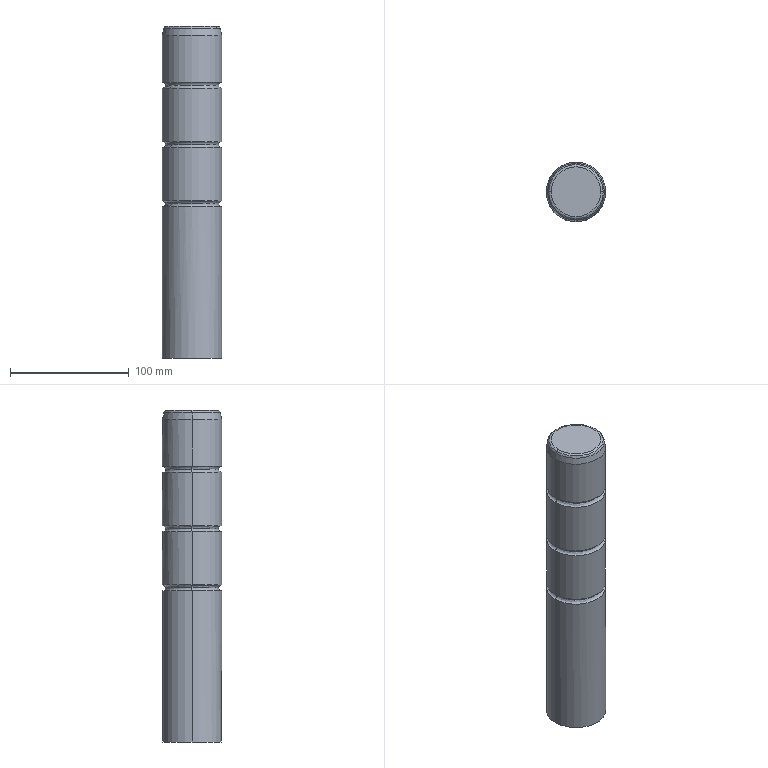Part | Creo | 1 solid | 33 faces | box 50 x 50 x 280 mm | volume 542043 mm3 | torus 16 | cylinder 10 | cone 4 | plane 3 | commonest cylinder face diameters 50 x8 10.579 x2
STEP:
#1=CARTESIAN_POINT('',(0.,0.,0.));
#2=DIRECTION('',(0.,0.,1.));
#3=DIRECTION('',(1.,0.,0.));
#4=AXIS2_PLACEMENT_3D('',#1,#2,#3);
#5=CARTESIAN_POINT('',(-257.899,252.373,-128.441));
#6=VERTEX_POINT('',#5);
#7=CARTESIAN_POINT('',(-307.899,252.373,-128.441));
#8=VERTEX_POINT('',#7);
#9=CARTESIAN_POINT('',(-282.899,252.373,-128.441));
#10=DIRECTION('',(0.,0.,-1.));
#11=DIRECTION('',(1.,0.,0.));
#12=AXIS2_PLACEMENT_3D('',#9,#10,#11);
#13=CIRCLE('',#12,25.);
#14=EDGE_CURVE('',#6,#8,#13,.T.);
#15=ORIENTED_EDGE('',*,*,#14,.F.);
#16=CARTESIAN_POINT('',(-282.899,252.373,-128.441));
#17=DIRECTION('',(0.,0.,-1.));
#18=DIRECTION('',(-1.,0.,0.));
#19=AXIS2_PLACEMENT_3D('',#16,#17,#18);
#20=CIRCLE('',#19,25.);
#21=EDGE_CURVE('',#8,#6,#20,.T.);
#22=ORIENTED_EDGE('',*,*,#21,.F.);
#23=EDGE_LOOP('',(#15,#22));
#24=FACE_OUTER_BOUND('',#23,.F.);
#25=CARTESIAN_POINT('',(-282.899,257.662,-128.441));
#26=VERTEX_POINT('',#25);
#27=CARTESIAN_POINT('',(-288.189,252.373,-128.441));
#28=VERTEX_POINT('',#27);
#29=CARTESIAN_POINT('',(-282.899,252.373,-128.441));
#30=DIRECTION('',(0.,0.,1.));
#31=DIRECTION('',(0.,1.,0.));
#32=AXIS2_PLACEMENT_3D('',#29,#30,#31);
#33=CIRCLE('',#32,5.29);
#34=EDGE_CURVE('',#26,#28,#33,.T.);
#35=ORIENTED_EDGE('',*,*,#34,.F.);
#36=CARTESIAN_POINT('',(-277.61,252.373,-128.441));
#37=VERTEX_POINT('',#36);
#38=CARTESIAN_POINT('',(-282.899,252.373,-128.441));
#39=DIRECTION('',(0.,0.,1.));
#40=DIRECTION('',(1.,0.,0.));
#41=AXIS2_PLACEMENT_3D('',#38,#39,#40);
#42=CIRCLE('',#41,5.29);
#43=EDGE_CURVE('',#37,#26,#42,.T.);
#44=ORIENTED_EDGE('',*,*,#43,.F.);
#45=CARTESIAN_POINT('',(-282.899,252.373,-128.441));
#46=DIRECTION('',(0.,0.,1.));
#47=DIRECTION('',(-1.,0.,0.));
#48=AXIS2_PLACEMENT_3D('',#45,#46,#47);
#49=CIRCLE('',#48,5.29);
#50=EDGE_CURVE('',#28,#37,#49,.T.);
#51=ORIENTED_EDGE('',*,*,#50,.F.);
#52=EDGE_LOOP('',(#35,#44,#51));
#53=FACE_BOUND('',#52,.F.);
#54=CARTESIAN_POINT('',(71.601,-52.127,-128.441));
#55=DIRECTION('',(0.,0.,-1.));
#56=DIRECTION('',(-1.,0.,0.));
#57=AXIS2_PLACEMENT_3D('',#54,#55,#56);
#58=PLANE('',#57);
#59=ADVANCED_FACE('',(#24,#53),#58,.T.);
#60=ORIENTED_EDGE('',*,*,#43,.T.);
#61=ORIENTED_EDGE('',*,*,#34,.T.);
#62=CARTESIAN_POINT('',(-288.189,252.373,-104.441));
#63=VERTEX_POINT('',#62);
#64=CARTESIAN_POINT('',(-288.189,252.373,-128.441));
#65=DIRECTION('',(0.,0.,1.));
#66=VECTOR('',#65,24.);
#67=LINE('',#64,#66);
#68=EDGE_CURVE('',#28,#63,#67,.T.);
#69=ORIENTED_EDGE('',*,*,#68,.T.);
#70=CARTESIAN_POINT('',(-282.899,257.662,-104.441));
#71=VERTEX_POINT('',#70);
#72=CARTESIAN_POINT('',(-282.899,252.373,-104.441));
#73=DIRECTION('',(0.,0.,-1.));
#74=DIRECTION('',(-1.,0.,0.));
#75=AXIS2_PLACEMENT_3D('',#72,#73,#74);
#76=CIRCLE('',#75,5.29);
#77=EDGE_CURVE('',#63,#71,#76,.T.);
#78=ORIENTED_EDGE('',*,*,#77,.T.);
#79=CARTESIAN_POINT('',(-277.61,252.373,-104.441));
#80=VERTEX_POINT('',#79);
#81=CARTESIAN_POINT('',(-282.899,252.373,-104.441));
#82=DIRECTION('',(0.,0.,-1.));
#83=DIRECTION('',(0.,1.,0.));
#84=AXIS2_PLACEMENT_3D('',#81,#82,#83);
#85=CIRCLE('',#84,5.29);
#86=EDGE_CURVE('',#71,#80,#85,.T.);
#87=ORIENTED_EDGE('',*,*,#86,.T.);
#88=CARTESIAN_POINT('',(-277.61,252.373,-128.441));
#89=DIRECTION('',(0.,0.,1.));
#90=VECTOR('',#89,24.);
#91=LINE('',#88,#90);
#92=EDGE_CURVE('',#37,#80,#91,.T.);
#93=ORIENTED_EDGE('',*,*,#92,.F.);
#94=EDGE_LOOP('',(#60,#61,#69,#78,#87,#93));
#95=FACE_OUTER_BOUND('',#94,.F.);
#96=CARTESIAN_POINT('',(-282.899,252.373,-215.441));
#97=DIRECTION('',(0.,0.,1.));
#98=DIRECTION('',(1.,0.,0.));
#99=AXIS2_PLACEMENT_3D('',#96,#97,#98);
#100=CYLINDRICAL_SURFACE('',#99,5.29);
#101=ADVANCED_FACE('',(#95),#100,.F.);
#102=ORIENTED_EDGE('',*,*,#50,.T.);
#103=ORIENTED_EDGE('',*,*,#92,.T.);
#104=CARTESIAN_POINT('',(-282.899,252.373,-104.441));
#105=DIRECTION('',(0.,0.,-1.));
#106=DIRECTION('',(1.,0.,0.));
#107=AXIS2_PLACEMENT_3D('',#104,#105,#106);
#108=CIRCLE('',#107,5.29);
#109=EDGE_CURVE('',#80,#63,#108,.T.);
#110=ORIENTED_EDGE('',*,*,#109,.T.);
#111=ORIENTED_EDGE('',*,*,#68,.F.);
#112=EDGE_LOOP('',(#102,#103,#110,#111));
#113=FACE_OUTER_BOUND('',#112,.F.);
#114=CARTESIAN_POINT('',(-282.899,252.373,-215.441));
#115=DIRECTION('',(0.,0.,1.));
#116=DIRECTION('',(1.,0.,0.));
#117=AXIS2_PLACEMENT_3D('',#114,#115,#116);
#118=CYLINDRICAL_SURFACE('',#117,5.29);
#119=ADVANCED_FACE('',(#113),#118,.F.);
#120=CARTESIAN_POINT('',(-282.899,252.12,-101.415));
#121=VERTEX_POINT('',#120);
#122=CARTESIAN_POINT('',(-283.152,252.373,-101.415));
#123=VERTEX_POINT('',#122);
#124=CARTESIAN_POINT('',(-282.899,252.373,-101.415));
#125=DIRECTION('',(0.,0.,-1.));
#126=DIRECTION('',(0.,-1.,0.));
#127=AXIS2_PLACEMENT_3D('',#124,#125,#126);
#128=CIRCLE('',#127,0.2524);
#129=EDGE_CURVE('',#121,#123,#128,.T.);
#130=ORIENTED_EDGE('',*,*,#129,.T.);
#131=CARTESIAN_POINT('',(-283.152,252.373,-101.415));
#132=DIRECTION('',(-0.8572,0.,-0.515));
#133=VECTOR('',#132,5.877);
#134=LINE('',#131,#133);
#135=EDGE_CURVE('',#123,#63,#134,.T.);
#136=ORIENTED_EDGE('',*,*,#135,.T.);
#137=ORIENTED_EDGE('',*,*,#109,.F.);
#138=CARTESIAN_POINT('',(-282.647,252.373,-101.415));
#139=VERTEX_POINT('',#138);
#140=CARTESIAN_POINT('',(-282.647,252.373,-101.415));
#141=DIRECTION('',(0.8572,0.,-0.515));
#142=VECTOR('',#141,5.877);
#143=LINE('',#140,#142);
#144=EDGE_CURVE('',#139,#80,#143,.T.);
#145=ORIENTED_EDGE('',*,*,#144,.F.);
#146=CARTESIAN_POINT('',(-282.899,252.373,-101.415));
#147=DIRECTION('',(0.,0.,-1.));
#148=DIRECTION('',(1.,0.,0.));
#149=AXIS2_PLACEMENT_3D('',#146,#147,#148);
#150=CIRCLE('',#149,0.2524);
#151=EDGE_CURVE('',#139,#121,#150,.T.);
#152=ORIENTED_EDGE('',*,*,#151,.T.);
#153=EDGE_LOOP('',(#130,#136,#137,#145,#152));
#154=FACE_OUTER_BOUND('',#153,.F.);
#155=CARTESIAN_POINT('',(-282.899,252.373,-102.928));
#156=DIRECTION('',(0.,0.,-1.));
#157=DIRECTION('',(-1.,0.,0.));
#158=AXIS2_PLACEMENT_3D('',#155,#156,#157);
#159=CONICAL_SURFACE('',#158,2.771,59.);
#160=ADVANCED_FACE('',(#154),#159,.F.);
#161=CARTESIAN_POINT('',(-282.899,252.625,-101.415));
#162=VERTEX_POINT('',#161);
#163=CARTESIAN_POINT('',(-282.808,252.608,-101.415));
#164=VERTEX_POINT('',#163);
#165=CARTESIAN_POINT('',(-282.899,252.373,-101.415));
#166=DIRECTION('',(0.,0.,-1.));
#167=DIRECTION('',(0.,1.,0.));
#168=AXIS2_PLACEMENT_3D('',#165,#166,#167);
#169=CIRCLE('',#168,0.2524);
#170=EDGE_CURVE('',#162,#164,#169,.T.);
#171=ORIENTED_EDGE('',*,*,#170,.F.);
#172=CARTESIAN_POINT('',(-282.99,252.608,-101.415));
#173=VERTEX_POINT('',#172);
#174=CARTESIAN_POINT('',(-282.899,252.373,-101.415));
#175=DIRECTION('',(0.,0.,-1.));
#176=DIRECTION('',(-0.361,0.9326,0.));
#177=AXIS2_PLACEMENT_3D('',#174,#175,#176);
#178=CIRCLE('',#177,0.2524);
#179=EDGE_CURVE('',#173,#162,#178,.T.);
#180=ORIENTED_EDGE('',*,*,#179,.F.);
#181=CARTESIAN_POINT('',(-282.899,252.373,-101.415));
#182=DIRECTION('',(0.,0.,-1.));
#183=DIRECTION('',(-1.,0.,0.));
#184=AXIS2_PLACEMENT_3D('',#181,#182,#183);
#185=CIRCLE('',#184,0.2524);
#186=EDGE_CURVE('',#123,#173,#185,.T.);
#187=ORIENTED_EDGE('',*,*,#186,.F.);
#188=ORIENTED_EDGE('',*,*,#129,.F.);
#189=ORIENTED_EDGE('',*,*,#151,.F.);
#190=CARTESIAN_POINT('',(-282.899,252.373,-101.415));
#191=DIRECTION('',(0.,0.,-1.));
#192=DIRECTION('',(0.361,0.9326,0.));
#193=AXIS2_PLACEMENT_3D('',#190,#191,#192);
#194=CIRCLE('',#193,0.2524);
#195=EDGE_CURVE('',#164,#139,#194,.T.);
#196=ORIENTED_EDGE('',*,*,#195,.F.);
#197=EDGE_LOOP('',(#171,#180,#187,#188,#189,#196));
#198=FACE_OUTER_BOUND('',#197,.F.);
#199=CARTESIAN_POINT('',(-282.899,252.373,-101.415));
#200=DIRECTION('',(0.,0.,1.));
#201=DIRECTION('',(1.,0.,0.));
#202=AXIS2_PLACEMENT_3D('',#199,#200,#201);
#203=PLANE('',#202);
#204=ADVANCED_FACE('',(#198),#203,.F.);
#205=ORIENTED_EDGE('',*,*,#179,.T.);
#206=ORIENTED_EDGE('',*,*,#170,.T.);
#207=ORIENTED_EDGE('',*,*,#195,.T.);
#208=ORIENTED_EDGE('',*,*,#144,.T.);
#209=ORIENTED_EDGE('',*,*,#86,.F.);
#210=ORIENTED_EDGE('',*,*,#77,.F.);
#211=ORIENTED_EDGE('',*,*,#135,.F.);
#212=ORIENTED_EDGE('',*,*,#186,.T.);
#213=EDGE_LOOP('',(#205,#206,#207,#208,#209,#210,#211,#212));
#214=FACE_OUTER_BOUND('',#213,.F.);
#215=CARTESIAN_POINT('',(-282.899,252.373,-102.928));
#216=DIRECTION('',(0.,0.,-1.));
#217=DIRECTION('',(-1.,0.,0.));
#218=AXIS2_PLACEMENT_3D('',#215,#216,#217);
#219=CONICAL_SURFACE('',#218,2.771,59.);
#220=ADVANCED_FACE('',(#214),#219,.F.);
#221=CARTESIAN_POINT('',(-307.899,252.373,-0.9415));
#222=VERTEX_POINT('',#221);
#223=CARTESIAN_POINT('',(-282.899,227.373,-0.9415));
#224=VERTEX_POINT('',#223);
#225=CARTESIAN_POINT('',(-282.899,252.373,-0.9415));
#226=DIRECTION('',(0.,0.,1.));
#227=DIRECTION('',(-1.,0.,0.));
#228=AXIS2_PLACEMENT_3D('',#225,#226,#227);
#229=CIRCLE('',#228,25.);
#230=EDGE_CURVE('',#222,#224,#229,.T.);
#231=ORIENTED_EDGE('',*,*,#230,.T.);
#232=CARTESIAN_POINT('',(-257.899,252.373,-0.9415));
#233=VERTEX_POINT('',#232);
#234=CARTESIAN_POINT('',(-282.899,252.373,-0.9415));
#235=DIRECTION('',(0.,0.,1.));
#236=DIRECTION('',(0.,-1.,0.));
#237=AXIS2_PLACEMENT_3D('',#234,#235,#236);
#238=CIRCLE('',#237,25.);
#239=EDGE_CURVE('',#224,#233,#238,.T.);
#240=ORIENTED_EDGE('',*,*,#239,.T.);
#241=CARTESIAN_POINT('',(-257.899,252.373,-128.441));
#242=DIRECTION('',(0.,0.,1.));
#243=VECTOR('',#242,127.5);
#244=LINE('',#241,#243);
#245=EDGE_CURVE('',#6,#233,#244,.T.);
#246=ORIENTED_EDGE('',*,*,#245,.F.);
#247=ORIENTED_EDGE('',*,*,#14,.T.);
#248=CARTESIAN_POINT('',(-307.899,252.373,-128.441));
#249=DIRECTION('',(0.,0.,1.));
#250=VECTOR('',#249,127.5);
#251=LINE('',#248,#250);
#252=EDGE_CURVE('',#8,#222,#251,.T.);
#253=ORIENTED_EDGE('',*,*,#252,.T.);
#254=EDGE_LOOP('',(#231,#240,#246,#247,#253));
#255=FACE_OUTER_BOUND('',#254,.F.);
#256=CARTESIAN_POINT('',(-282.899,252.373,-216.441));
#257=DIRECTION('',(0.,0.,1.));
#258=DIRECTION('',(1.,0.,0.));
#259=AXIS2_PLACEMENT_3D('',#256,#257,#258);
#260=CYLINDRICAL_SURFACE('',#259,25.);
#261=ADVANCED_FACE('',(#255),#260,.T.);
#262=ORIENTED_EDGE('',*,*,#239,.F.);
#263=ORIENTED_EDGE('',*,*,#230,.F.);
#264=CARTESIAN_POINT('',(-305.399,252.373,1.559));
#265=VERTEX_POINT('',#264);
#266=CARTESIAN_POINT('',(-307.899,252.373,1.559));
#267=DIRECTION('',(0.,1.,0.));
#268=DIRECTION('',(1.,0.,0.));
#269=AXIS2_PLACEMENT_3D('',#266,#267,#268);
#270=CIRCLE('',#269,2.5);
#271=EDGE_CURVE('',#265,#222,#270,.T.);
#272=ORIENTED_EDGE('',*,*,#271,.F.);
#273=CARTESIAN_POINT('',(-260.399,252.373,1.559));
#274=VERTEX_POINT('',#273);
#275=CARTESIAN_POINT('',(-282.899,252.373,1.559));
#276=DIRECTION('',(0.,0.,1.));
#277=DIRECTION('',(-1.,0.,0.));
#278=AXIS2_PLACEMENT_3D('',#275,#276,#277);
#279=CIRCLE('',#278,22.5);
#280=EDGE_CURVE('',#265,#274,#279,.T.);
#281=ORIENTED_EDGE('',*,*,#280,.T.);
#282=CARTESIAN_POINT('',(-257.899,252.373,1.559));
#283=DIRECTION('',(0.,-1.,0.));
#284=DIRECTION('',(-1.,0.,0.));
#285=AXIS2_PLACEMENT_3D('',#282,#283,#284);
#286=CIRCLE('',#285,2.5);
#287=EDGE_CURVE('',#274,#233,#286,.T.);
#288=ORIENTED_EDGE('',*,*,#287,.T.);
#289=EDGE_LOOP('',(#262,#263,#272,#281,#288));
#290=FACE_OUTER_BOUND('',#289,.F.);
#291=CARTESIAN_POINT('',(-282.899,252.373,1.559));
#292=DIRECTION('',(0.,0.,1.));
#293=DIRECTION('',(1.,0.,0.));
#294=AXIS2_PLACEMENT_3D('',#291,#292,#293);
#295=TOROIDAL_SURFACE('',#294,25.,2.5);
#296=ADVANCED_FACE('',(#290),#295,.F.);
#297=CARTESIAN_POINT('',(-282.899,252.373,-0.9415));
#298=DIRECTION('',(0.,0.,1.));
#299=DIRECTION('',(1.,0.,0.));
#300=AXIS2_PLACEMENT_3D('',#297,#298,#299);
#301=CIRCLE('',#300,25.);
#302=EDGE_CURVE('',#233,#222,#301,.T.);
#303=ORIENTED_EDGE('',*,*,#302,.F.);
#304=ORIENTED_EDGE('',*,*,#287,.F.);
#305=CARTESIAN_POINT('',(-282.899,252.373,1.559));
#306=DIRECTION('',(0.,0.,1.));
#307=DIRECTION('',(1.,0.,0.));
#308=AXIS2_PLACEMENT_3D('',#305,#306,#307);
#309=CIRCLE('',#308,22.5);
#310=EDGE_CURVE('',#274,#265,#309,.T.);
#311=ORIENTED_EDGE('',*,*,#310,.T.);
#312=ORIENTED_EDGE('',*,*,#271,.T.);
#313=EDGE_LOOP('',(#303,#304,#311,#312));
#314=FACE_OUTER_BOUND('',#313,.F.);
#315=CARTESIAN_POINT('',(-282.899,252.373,1.559));
#316=DIRECTION('',(0.,0.,1.));
#317=DIRECTION('',(1.,0.,0.));
#318=AXIS2_PLACEMENT_3D('',#315,#316,#317);
#319=TOROIDAL_SURFACE('',#318,25.,2.5);
#320=ADVANCED_FACE('',(#314),#319,.F.);
#321=ORIENTED_EDGE('',*,*,#302,.T.);
#322=ORIENTED_EDGE('',*,*,#252,.F.);
#323=ORIENTED_EDGE('',*,*,#21,.T.);
#324=ORIENTED_EDGE('',*,*,#245,.T.);
#325=EDGE_LOOP('',(#321,#322,#323,#324));
#326=FACE_OUTER_BOUND('',#325,.F.);
#327=CARTESIAN_POINT('',(-282.899,252.373,-216.441));
#328=DIRECTION('',(0.,0.,1.));
#329=DIRECTION('',(1.,0.,0.));
#330=AXIS2_PLACEMENT_3D('',#327,#328,#329);
#331=CYLINDRICAL_SURFACE('',#330,25.);
#332=ADVANCED_FACE('',(#326),#331,.T.);
#333=CARTESIAN_POINT('',(-307.899,252.373,4.059));
#334=VERTEX_POINT('',#333);
#335=CARTESIAN_POINT('',(-282.899,277.373,4.059));
#336=VERTEX_POINT('',#335);
#337=CARTESIAN_POINT('',(-282.899,252.373,4.059));
#338=DIRECTION('',(0.,0.,-1.));
#339=DIRECTION('',(-1.,0.,0.));
#340=AXIS2_PLACEMENT_3D('',#337,#338,#339);
#341=CIRCLE('',#340,25.);
#342=EDGE_CURVE('',#334,#336,#341,.T.);
#343=ORIENTED_EDGE('',*,*,#342,.F.);
#344=CARTESIAN_POINT('',(-307.899,252.373,1.559));
#345=DIRECTION('',(0.,1.,0.));
#346=DIRECTION('',(0.,0.,1.));
#347=AXIS2_PLACEMENT_3D('',#344,#345,#346);
#348=CIRCLE('',#347,2.5);
#349=EDGE_CURVE('',#334,#265,#348,.T.);
#350=ORIENTED_EDGE('',*,*,#349,.T.);
#351=ORIENTED_EDGE('',*,*,#310,.F.);
#352=CARTESIAN_POINT('',(-257.899,252.373,4.059));
#353=VERTEX_POINT('',#352);
#354=CARTESIAN_POINT('',(-257.899,252.373,1.559));
#355=DIRECTION('',(0.,-1.,0.));
#356=DIRECTION('',(0.,0.,1.));
#357=AXIS2_PLACEMENT_3D('',#354,#355,#356);
#358=CIRCLE('',#357,2.5);
#359=EDGE_CURVE('',#353,#274,#358,.T.);
#360=ORIENTED_EDGE('',*,*,#359,.F.);
#361=CARTESIAN_POINT('',(-282.899,252.373,4.059));
#362=DIRECTION('',(0.,0.,-1.));
#363=DIRECTION('',(0.,1.,0.));
#364=AXIS2_PLACEMENT_3D('',#361,#362,#363);
#365=CIRCLE('',#364,25.);
#366=EDGE_CURVE('',#336,#353,#365,.T.);
#367=ORIENTED_EDGE('',*,*,#366,.F.);
#368=EDGE_LOOP('',(#343,#350,#351,#360,#367));
#369=FACE_OUTER_BOUND('',#368,.F.);
#370=CARTESIAN_POINT('',(-282.899,252.373,1.559));
#371=DIRECTION('',(0.,0.,1.));
#372=DIRECTION('',(1.,0.,0.));
#373=AXIS2_PLACEMENT_3D('',#370,#371,#372);
#374=TOROIDAL_SURFACE('',#373,25.,2.5);
#375=ADVANCED_FACE('',(#369),#374,.F.);
#376=CARTESIAN_POINT('',(-257.899,252.373,49.059));
#377=VERTEX_POINT('',#376);
#378=CARTESIAN_POINT('',(-307.899,252.373,49.059));
#379=VERTEX_POINT('',#378);
#380=CARTESIAN_POINT('',(-282.899,252.373,49.059));
#381=DIRECTION('',(0.,0.,1.));
#382=DIRECTION('',(1.,0.,0.));
#383=AXIS2_PLACEMENT_3D('',#380,#381,#382);
#384=CIRCLE('',#383,25.);
#385=EDGE_CURVE('',#377,#379,#384,.T.);
#386=ORIENTED_EDGE('',*,*,#385,.T.);
#387=CARTESIAN_POINT('',(-307.899,252.373,4.059));
#388=DIRECTION('',(0.,0.,1.));
#389=VECTOR('',#388,45.);
#390=LINE('',#387,#389);
#391=EDGE_CURVE('',#334,#379,#390,.T.);
#392=ORIENTED_EDGE('',*,*,#391,.F.);
#393=ORIENTED_EDGE('',*,*,#342,.T.);
#394=ORIENTED_EDGE('',*,*,#366,.T.);
#395=CARTESIAN_POINT('',(-257.899,252.373,4.059));
#396=DIRECTION('',(0.,0.,1.));
#397=VECTOR('',#396,45.);
#398=LINE('',#395,#397);
#399=EDGE_CURVE('',#353,#377,#398,.T.);
#400=ORIENTED_EDGE('',*,*,#399,.T.);
#401=EDGE_LOOP('',(#386,#392,#393,#394,#400));
#402=FACE_OUTER_BOUND('',#401,.F.);
#403=CARTESIAN_POINT('',(-282.899,252.373,-216.441));
#404=DIRECTION('',(0.,0.,1.));
#405=DIRECTION('',(1.,0.,0.));
#406=AXIS2_PLACEMENT_3D('',#403,#404,#405);
#407=CYLINDRICAL_SURFACE('',#406,25.);
#408=ADVANCED_FACE('',(#402),#407,.T.);
#409=ORIENTED_EDGE('',*,*,#385,.F.);
#410=CARTESIAN_POINT('',(-260.399,252.373,51.559));
#411=VERTEX_POINT('',#410);
#412=CARTESIAN_POINT('',(-257.899,252.373,51.559));
#413=DIRECTION('',(0.,-1.,0.));
#414=DIRECTION('',(-1.,0.,0.));
#415=AXIS2_PLACEMENT_3D('',#412,#413,#414);
#416=CIRCLE('',#415,2.5);
#417=EDGE_CURVE('',#411,#377,#416,.T.);
#418=ORIENTED_EDGE('',*,*,#417,.F.);
#419=CARTESIAN_POINT('',(-305.399,252.373,51.559));
#420=VERTEX_POINT('',#419);
#421=CARTESIAN_POINT('',(-282.899,252.373,51.559));
#422=DIRECTION('',(0.,0.,1.));
#423=DIRECTION('',(1.,0.,0.));
#424=AXIS2_PLACEMENT_3D('',#421,#422,#423);
#425=CIRCLE('',#424,22.5);
#426=EDGE_CURVE('',#411,#420,#425,.T.);
#427=ORIENTED_EDGE('',*,*,#426,.T.);
#428=CARTESIAN_POINT('',(-307.899,252.373,51.559));
#429=DIRECTION('',(0.,1.,0.));
#430=DIRECTION('',(1.,0.,0.));
#431=AXIS2_PLACEMENT_3D('',#428,#429,#430);
#432=CIRCLE('',#431,2.5);
#433=EDGE_CURVE('',#420,#379,#432,.T.);
#434=ORIENTED_EDGE('',*,*,#433,.T.);
#435=EDGE_LOOP('',(#409,#418,#427,#434));
#436=FACE_OUTER_BOUND('',#435,.F.);
#437=CARTESIAN_POINT('',(-282.899,252.373,51.559));
#438=DIRECTION('',(0.,0.,1.));
#439=DIRECTION('',(1.,0.,0.));
#440=AXIS2_PLACEMENT_3D('',#437,#438,#439);
#441=TOROIDAL_SURFACE('',#440,25.,2.5);
#442=ADVANCED_FACE('',(#436),#441,.F.);
#443=CARTESIAN_POINT('',(-282.899,227.373,49.059));
#444=VERTEX_POINT('',#443);
#445=CARTESIAN_POINT('',(-282.899,252.373,49.059));
#446=DIRECTION('',(0.,0.,1.));
#447=DIRECTION('',(0.,-1.,0.));
#448=AXIS2_PLACEMENT_3D('',#445,#446,#447);
#449=CIRCLE('',#448,25.);
#450=EDGE_CURVE('',#444,#377,#449,.T.);
#451=ORIENTED_EDGE('',*,*,#450,.F.);
#452=CARTESIAN_POINT('',(-282.899,252.373,49.059));
#453=DIRECTION('',(0.,0.,1.));
#454=DIRECTION('',(-1.,0.,0.));
#455=AXIS2_PLACEMENT_3D('',#452,#453,#454);
#456=CIRCLE('',#455,25.);
#457=EDGE_CURVE('',#379,#444,#456,.T.);
#458=ORIENTED_EDGE('',*,*,#457,.F.);
#459=ORIENTED_EDGE('',*,*,#433,.F.);
#460=CARTESIAN_POINT('',(-282.899,252.373,51.559));
#461=DIRECTION('',(0.,0.,1.));
#462=DIRECTION('',(-1.,0.,0.));
#463=AXIS2_PLACEMENT_3D('',#460,#461,#462);
#464=CIRCLE('',#463,22.5);
#465=EDGE_CURVE('',#420,#411,#464,.T.);
#466=ORIENTED_EDGE('',*,*,#465,.T.);
#467=ORIENTED_EDGE('',*,*,#417,.T.);
#468=EDGE_LOOP('',(#451,#458,#459,#466,#467));
#469=FACE_OUTER_BOUND('',#468,.F.);
#470=CARTESIAN_POINT('',(-282.899,252.373,51.559));
#471=DIRECTION('',(0.,0.,1.));
#472=DIRECTION('',(1.,0.,0.));
#473=AXIS2_PLACEMENT_3D('',#470,#471,#472);
#474=TOROIDAL_SURFACE('',#473,25.,2.5);
#475=ADVANCED_FACE('',(#469),#474,.F.);
#476=ORIENTED_EDGE('',*,*,#457,.T.);
#477=ORIENTED_EDGE('',*,*,#450,.T.);
#478=ORIENTED_EDGE('',*,*,#399,.F.);
#479=CARTESIAN_POINT('',(-282.899,227.373,4.059));
#480=VERTEX_POINT('',#479);
#481=CARTESIAN_POINT('',(-282.899,252.373,4.059));
#482=DIRECTION('',(0.,0.,-1.));
#483=DIRECTION('',(1.,0.,0.));
#484=AXIS2_PLACEMENT_3D('',#481,#482,#483);
#485=CIRCLE('',#484,25.);
#486=EDGE_CURVE('',#353,#480,#485,.T.);
#487=ORIENTED_EDGE('',*,*,#486,.T.);
#488=CARTESIAN_POINT('',(-282.899,252.373,4.059));
#489=DIRECTION('',(0.,0.,-1.));
#490=DIRECTION('',(0.,-1.,0.));
#491=AXIS2_PLACEMENT_3D('',#488,#489,#490);
#492=CIRCLE('',#491,25.);
#493=EDGE_CURVE('',#480,#334,#492,.T.);
#494=ORIENTED_EDGE('',*,*,#493,.T.);
#495=ORIENTED_EDGE('',*,*,#391,.T.);
#496=EDGE_LOOP('',(#476,#477,#478,#487,#494,#495));
#497=FACE_OUTER_BOUND('',#496,.F.);
#498=CARTESIAN_POINT('',(-282.899,252.373,-216.441));
#499=DIRECTION('',(0.,0.,1.));
#500=DIRECTION('',(1.,0.,0.));
#501=AXIS2_PLACEMENT_3D('',#498,#499,#500);
#502=CYLINDRICAL_SURFACE('',#501,25.);
#503=ADVANCED_FACE('',(#497),#502,.T.);
#504=ORIENTED_EDGE('',*,*,#493,.F.);
#505=ORIENTED_EDGE('',*,*,#486,.F.);
#506=ORIENTED_EDGE('',*,*,#359,.T.);
#507=ORIENTED_EDGE('',*,*,#280,.F.);
#508=ORIENTED_EDGE('',*,*,#349,.F.);
#509=EDGE_LOOP('',(#504,#505,#506,#507,#508));
#510=FACE_OUTER_BOUND('',#509,.F.);
#511=CARTESIAN_POINT('',(-282.899,252.373,1.559));
#512=DIRECTION('',(0.,0.,1.));
#513=DIRECTION('',(1.,0.,0.));
#514=AXIS2_PLACEMENT_3D('',#511,#512,#513);
#515=TOROIDAL_SURFACE('',#514,25.,2.5);
#516=ADVANCED_FACE('',(#510),#515,.F.);
#517=CARTESIAN_POINT('',(-282.899,227.373,54.059));
#518=VERTEX_POINT('',#517);
#519=CARTESIAN_POINT('',(-307.899,252.373,54.059));
#520=VERTEX_POINT('',#519);
#521=CARTESIAN_POINT('',(-282.899,252.373,54.059));
#522=DIRECTION('',(0.,0.,-1.));
#523=DIRECTION('',(0.,-1.,0.));
#524=AXIS2_PLACEMENT_3D('',#521,#522,#523);
#525=CIRCLE('',#524,25.);
#526=EDGE_CURVE('',#518,#520,#525,.T.);
#527=ORIENTED_EDGE('',*,*,#526,.F.);
#528=CARTESIAN_POINT('',(-257.899,252.373,54.059));
#529=VERTEX_POINT('',#528);
#530=CARTESIAN_POINT('',(-282.899,252.373,54.059));
#531=DIRECTION('',(0.,0.,-1.));
#532=DIRECTION('',(1.,0.,0.));
#533=AXIS2_PLACEMENT_3D('',#530,#531,#532);
#534=CIRCLE('',#533,25.);
#535=EDGE_CURVE('',#529,#518,#534,.T.);
#536=ORIENTED_EDGE('',*,*,#535,.F.);
#537=CARTESIAN_POINT('',(-257.899,252.373,51.559));
#538=DIRECTION('',(0.,-1.,0.));
#539=DIRECTION('',(0.,0.,1.));
#540=AXIS2_PLACEMENT_3D('',#537,#538,#539);
#541=CIRCLE('',#540,2.5);
#542=EDGE_CURVE('',#529,#411,#541,.T.);
#543=ORIENTED_EDGE('',*,*,#542,.T.);
#544=ORIENTED_EDGE('',*,*,#465,.F.);
#545=CARTESIAN_POINT('',(-307.899,252.373,51.559));
#546=DIRECTION('',(0.,1.,0.));
#547=DIRECTION('',(0.,0.,1.));
#548=AXIS2_PLACEMENT_3D('',#545,#546,#547);
#549=CIRCLE('',#548,2.5);
#550=EDGE_CURVE('',#520,#420,#549,.T.);
#551=ORIENTED_EDGE('',*,*,#550,.F.);
#552=EDGE_LOOP('',(#527,#536,#543,#544,#551));
#553=FACE_OUTER_BOUND('',#552,.F.);
#554=CARTESIAN_POINT('',(-282.899,252.373,51.559));
#555=DIRECTION('',(0.,0.,1.));
#556=DIRECTION('',(1.,0.,0.));
#557=AXIS2_PLACEMENT_3D('',#554,#555,#556);
#558=TOROIDAL_SURFACE('',#557,25.,2.5);
#559=ADVANCED_FACE('',(#553),#558,.F.);
#560=CARTESIAN_POINT('',(-307.899,252.373,99.059));
#561=VERTEX_POINT('',#560);
#562=CARTESIAN_POINT('',(-282.899,227.373,99.059));
#563=VERTEX_POINT('',#562);
#564=CARTESIAN_POINT('',(-282.899,252.373,99.059));
#565=DIRECTION('',(0.,0.,1.));
#566=DIRECTION('',(-1.,0.,0.));
#567=AXIS2_PLACEMENT_3D('',#564,#565,#566);
#568=CIRCLE('',#567,25.);
#569=EDGE_CURVE('',#561,#563,#568,.T.);
#570=ORIENTED_EDGE('',*,*,#569,.T.);
#571=CARTESIAN_POINT('',(-257.899,252.373,99.059));
#572=VERTEX_POINT('',#571);
#573=CARTESIAN_POINT('',(-282.899,252.373,99.059));
#574=DIRECTION('',(0.,0.,1.));
#575=DIRECTION('',(0.,-1.,0.));
#576=AXIS2_PLACEMENT_3D('',#573,#574,#575);
#577=CIRCLE('',#576,25.);
#578=EDGE_CURVE('',#563,#572,#577,.T.);
#579=ORIENTED_EDGE('',*,*,#578,.T.);
#580=CARTESIAN_POINT('',(-257.899,252.373,54.059));
#581=DIRECTION('',(0.,0.,1.));
#582=VECTOR('',#581,45.);
#583=LINE('',#580,#582);
#584=EDGE_CURVE('',#529,#572,#583,.T.);
#585=ORIENTED_EDGE('',*,*,#584,.F.);
#586=ORIENTED_EDGE('',*,*,#535,.T.);
#587=ORIENTED_EDGE('',*,*,#526,.T.);
#588=CARTESIAN_POINT('',(-307.899,252.373,54.059));
#589=DIRECTION('',(0.,0.,1.));
#590=VECTOR('',#589,45.);
#591=LINE('',#588,#590);
#592=EDGE_CURVE('',#520,#561,#591,.T.);
#593=ORIENTED_EDGE('',*,*,#592,.T.);
#594=EDGE_LOOP('',(#570,#579,#585,#586,#587,#593));
#595=FACE_OUTER_BOUND('',#594,.F.);
#596=CARTESIAN_POINT('',(-282.899,252.373,-216.441));
#597=DIRECTION('',(0.,0.,1.));
#598=DIRECTION('',(1.,0.,0.));
#599=AXIS2_PLACEMENT_3D('',#596,#597,#598);
#600=CYLINDRICAL_SURFACE('',#599,25.);
#601=ADVANCED_FACE('',(#595),#600,.T.);
#602=ORIENTED_EDGE('',*,*,#578,.F.);
#603=ORIENTED_EDGE('',*,*,#569,.F.);
#604=CARTESIAN_POINT('',(-305.399,252.373,101.559));
#605=VERTEX_POINT('',#604);
#606=CARTESIAN_POINT('',(-307.899,252.373,101.559));
#607=DIRECTION('',(0.,1.,0.));
#608=DIRECTION('',(1.,0.,0.));
#609=AXIS2_PLACEMENT_3D('',#606,#607,#608);
#610=CIRCLE('',#609,2.5);
#611=EDGE_CURVE('',#605,#561,#610,.T.);
#612=ORIENTED_EDGE('',*,*,#611,.F.);
#613=CARTESIAN_POINT('',(-260.399,252.373,101.559));
#614=VERTEX_POINT('',#613);
#615=CARTESIAN_POINT('',(-282.899,252.373,101.559));
#616=DIRECTION('',(0.,0.,1.));
#617=DIRECTION('',(-1.,0.,0.));
#618=AXIS2_PLACEMENT_3D('',#615,#616,#617);
#619=CIRCLE('',#618,22.5);
#620=EDGE_CURVE('',#605,#614,#619,.T.);
#621=ORIENTED_EDGE('',*,*,#620,.T.);
#622=CARTESIAN_POINT('',(-257.899,252.373,101.559));
#623=DIRECTION('',(0.,-1.,0.));
#624=DIRECTION('',(-1.,0.,0.));
#625=AXIS2_PLACEMENT_3D('',#622,#623,#624);
#626=CIRCLE('',#625,2.5);
#627=EDGE_CURVE('',#614,#572,#626,.T.);
#628=ORIENTED_EDGE('',*,*,#627,.T.);
#629=EDGE_LOOP('',(#602,#603,#612,#621,#628));
#630=FACE_OUTER_BOUND('',#629,.F.);
#631=CARTESIAN_POINT('',(-282.899,252.373,101.559));
#632=DIRECTION('',(0.,0.,1.));
#633=DIRECTION('',(1.,0.,0.));
#634=AXIS2_PLACEMENT_3D('',#631,#632,#633);
#635=TOROIDAL_SURFACE('',#634,25.,2.5);
#636=ADVANCED_FACE('',(#630),#635,.F.);
#637=CARTESIAN_POINT('',(-282.899,252.373,99.059));
#638=DIRECTION('',(0.,0.,1.));
#639=DIRECTION('',(1.,0.,0.));
#640=AXIS2_PLACEMENT_3D('',#637,#638,#639);
#641=CIRCLE('',#640,25.);
#642=EDGE_CURVE('',#572,#561,#641,.T.);
#643=ORIENTED_EDGE('',*,*,#642,.F.);
#644=ORIENTED_EDGE('',*,*,#627,.F.);
#645=CARTESIAN_POINT('',(-282.899,252.373,101.559));
#646=DIRECTION('',(0.,0.,1.));
#647=DIRECTION('',(1.,0.,0.));
#648=AXIS2_PLACEMENT_3D('',#645,#646,#647);
#649=CIRCLE('',#648,22.5);
#650=EDGE_CURVE('',#614,#605,#649,.T.);
#651=ORIENTED_EDGE('',*,*,#650,.T.);
#652=ORIENTED_EDGE('',*,*,#611,.T.);
#653=EDGE_LOOP('',(#643,#644,#651,#652));
#654=FACE_OUTER_BOUND('',#653,.F.);
#655=CARTESIAN_POINT('',(-282.899,252.373,101.559));
#656=DIRECTION('',(0.,0.,1.));
#657=DIRECTION('',(1.,0.,0.));
#658=AXIS2_PLACEMENT_3D('',#655,#656,#657);
#659=TOROIDAL_SURFACE('',#658,25.,2.5);
#660=ADVANCED_FACE('',(#654),#659,.F.);
#661=ORIENTED_EDGE('',*,*,#642,.T.);
#662=ORIENTED_EDGE('',*,*,#592,.F.);
#663=CARTESIAN_POINT('',(-282.899,277.373,54.059));
#664=VERTEX_POINT('',#663);
#665=CARTESIAN_POINT('',(-282.899,252.373,54.059));
#666=DIRECTION('',(0.,0.,-1.));
#667=DIRECTION('',(-1.,0.,0.));
#668=AXIS2_PLACEMENT_3D('',#665,#666,#667);
#669=CIRCLE('',#668,25.);
#670=EDGE_CURVE('',#520,#664,#669,.T.);
#671=ORIENTED_EDGE('',*,*,#670,.T.);
#672=CARTESIAN_POINT('',(-282.899,252.373,54.059));
#673=DIRECTION('',(0.,0.,-1.));
#674=DIRECTION('',(0.,1.,0.));
#675=AXIS2_PLACEMENT_3D('',#672,#673,#674);
#676=CIRCLE('',#675,25.);
#677=EDGE_CURVE('',#664,#529,#676,.T.);
#678=ORIENTED_EDGE('',*,*,#677,.T.);
#679=ORIENTED_EDGE('',*,*,#584,.T.);
#680=EDGE_LOOP('',(#661,#662,#671,#678,#679));
#681=FACE_OUTER_BOUND('',#680,.F.);
#682=CARTESIAN_POINT('',(-282.899,252.373,-216.441));
#683=DIRECTION('',(0.,0.,1.));
#684=DIRECTION('',(1.,0.,0.));
#685=AXIS2_PLACEMENT_3D('',#682,#683,#684);
#686=CYLINDRICAL_SURFACE('',#685,25.);
#687=ADVANCED_FACE('',(#681),#686,.T.);
#688=ORIENTED_EDGE('',*,*,#670,.F.);
#689=ORIENTED_EDGE('',*,*,#550,.T.);
#690=ORIENTED_EDGE('',*,*,#426,.F.);
#691=ORIENTED_EDGE('',*,*,#542,.F.);
#692=ORIENTED_EDGE('',*,*,#677,.F.);
#693=EDGE_LOOP('',(#688,#689,#690,#691,#692));
#694=FACE_OUTER_BOUND('',#693,.F.);
#695=CARTESIAN_POINT('',(-282.899,252.373,51.559));
#696=DIRECTION('',(0.,0.,1.));
#697=DIRECTION('',(1.,0.,0.));
#698=AXIS2_PLACEMENT_3D('',#695,#696,#697);
#699=TOROIDAL_SURFACE('',#698,25.,2.5);
#700=ADVANCED_FACE('',(#694),#699,.F.);
#701=CARTESIAN_POINT('',(-307.899,252.373,104.059));
#702=VERTEX_POINT('',#701);
#703=CARTESIAN_POINT('',(-282.899,277.373,104.059));
#704=VERTEX_POINT('',#703);
#705=CARTESIAN_POINT('',(-282.899,252.373,104.059));
#706=DIRECTION('',(0.,0.,-1.));
#707=DIRECTION('',(-1.,0.,0.));
#708=AXIS2_PLACEMENT_3D('',#705,#706,#707);
#709=CIRCLE('',#708,25.);
#710=EDGE_CURVE('',#702,#704,#709,.T.);
#711=ORIENTED_EDGE('',*,*,#710,.F.);
#712=CARTESIAN_POINT('',(-307.899,252.373,101.559));
#713=DIRECTION('',(0.,1.,0.));
#714=DIRECTION('',(0.,0.,1.));
#715=AXIS2_PLACEMENT_3D('',#712,#713,#714);
#716=CIRCLE('',#715,2.5);
#717=EDGE_CURVE('',#702,#605,#716,.T.);
#718=ORIENTED_EDGE('',*,*,#717,.T.);
#719=ORIENTED_EDGE('',*,*,#650,.F.);
#720=CARTESIAN_POINT('',(-257.899,252.373,104.059));
#721=VERTEX_POINT('',#720);
#722=CARTESIAN_POINT('',(-257.899,252.373,101.559));
#723=DIRECTION('',(0.,-1.,0.));
#724=DIRECTION('',(0.,0.,1.));
#725=AXIS2_PLACEMENT_3D('',#722,#723,#724);
#726=CIRCLE('',#725,2.5);
#727=EDGE_CURVE('',#721,#614,#726,.T.);
#728=ORIENTED_EDGE('',*,*,#727,.F.);
#729=CARTESIAN_POINT('',(-282.899,252.373,104.059));
#730=DIRECTION('',(0.,0.,-1.));
#731=DIRECTION('',(0.,1.,0.));
#732=AXIS2_PLACEMENT_3D('',#729,#730,#731);
#733=CIRCLE('',#732,25.);
#734=EDGE_CURVE('',#704,#721,#733,.T.);
#735=ORIENTED_EDGE('',*,*,#734,.F.);
#736=EDGE_LOOP('',(#711,#718,#719,#728,#735));
#737=FACE_OUTER_BOUND('',#736,.F.);
#738=CARTESIAN_POINT('',(-282.899,252.373,101.559));
#739=DIRECTION('',(0.,0.,1.));
#740=DIRECTION('',(1.,0.,0.));
#741=AXIS2_PLACEMENT_3D('',#738,#739,#740);
#742=TOROIDAL_SURFACE('',#741,25.,2.5);
#743=ADVANCED_FACE('',(#737),#742,.F.);
#744=ORIENTED_EDGE('',*,*,#734,.T.);
#745=CARTESIAN_POINT('',(-257.899,252.373,143.559));
#746=VERTEX_POINT('',#745);
#747=CARTESIAN_POINT('',(-257.899,252.373,104.059));
#748=DIRECTION('',(0.,0.,1.));
#749=VECTOR('',#748,39.5);
#750=LINE('',#747,#749);
#751=EDGE_CURVE('',#721,#746,#750,.T.);
#752=ORIENTED_EDGE('',*,*,#751,.T.);
#753=CARTESIAN_POINT('',(-307.899,252.373,143.559));
#754=VERTEX_POINT('',#753);
#755=CARTESIAN_POINT('',(-282.899,252.373,143.559));
#756=DIRECTION('',(0.,0.,1.));
#757=DIRECTION('',(1.,0.,0.));
#758=AXIS2_PLACEMENT_3D('',#755,#756,#757);
#759=CIRCLE('',#758,25.);
#760=EDGE_CURVE('',#746,#754,#759,.T.);
#761=ORIENTED_EDGE('',*,*,#760,.T.);
#762=CARTESIAN_POINT('',(-307.899,252.373,104.059));
#763=DIRECTION('',(0.,0.,1.));
#764=VECTOR('',#763,39.5);
#765=LINE('',#762,#764);
#766=EDGE_CURVE('',#702,#754,#765,.T.);
#767=ORIENTED_EDGE('',*,*,#766,.F.);
#768=ORIENTED_EDGE('',*,*,#710,.T.);
#769=EDGE_LOOP('',(#744,#752,#761,#767,#768));
#770=FACE_OUTER_BOUND('',#769,.F.);
#771=CARTESIAN_POINT('',(-282.899,252.373,-216.441));
#772=DIRECTION('',(0.,0.,1.));
#773=DIRECTION('',(1.,0.,0.));
#774=AXIS2_PLACEMENT_3D('',#771,#772,#773);
#775=CYLINDRICAL_SURFACE('',#774,25.);
#776=ADVANCED_FACE('',(#770),#775,.T.);
#777=CARTESIAN_POINT('',(-282.899,227.373,104.059));
#778=VERTEX_POINT('',#777);
#779=CARTESIAN_POINT('',(-282.899,252.373,104.059));
#780=DIRECTION('',(0.,0.,-1.));
#781=DIRECTION('',(1.,0.,0.));
#782=AXIS2_PLACEMENT_3D('',#779,#780,#781);
#783=CIRCLE('',#782,25.);
#784=EDGE_CURVE('',#721,#778,#783,.T.);
#785=ORIENTED_EDGE('',*,*,#784,.T.);
#786=CARTESIAN_POINT('',(-282.899,252.373,104.059));
#787=DIRECTION('',(0.,0.,-1.));
#788=DIRECTION('',(0.,-1.,0.));
#789=AXIS2_PLACEMENT_3D('',#786,#787,#788);
#790=CIRCLE('',#789,25.);
#791=EDGE_CURVE('',#778,#702,#790,.T.);
#792=ORIENTED_EDGE('',*,*,#791,.T.);
#793=ORIENTED_EDGE('',*,*,#766,.T.);
#794=CARTESIAN_POINT('',(-282.899,227.373,143.559));
#795=VERTEX_POINT('',#794);
#796=CARTESIAN_POINT('',(-282.899,252.373,143.559));
#797=DIRECTION('',(0.,0.,1.));
#798=DIRECTION('',(-1.,0.,0.));
#799=AXIS2_PLACEMENT_3D('',#796,#797,#798);
#800=CIRCLE('',#799,25.);
#801=EDGE_CURVE('',#754,#795,#800,.T.);
#802=ORIENTED_EDGE('',*,*,#801,.T.);
#803=CARTESIAN_POINT('',(-282.899,252.373,143.559));
#804=DIRECTION('',(0.,0.,1.));
#805=DIRECTION('',(0.,-1.,0.));
#806=AXIS2_PLACEMENT_3D('',#803,#804,#805);
#807=CIRCLE('',#806,25.);
#808=EDGE_CURVE('',#795,#746,#807,.T.);
#809=ORIENTED_EDGE('',*,*,#808,.T.);
#810=ORIENTED_EDGE('',*,*,#751,.F.);
#811=EDGE_LOOP('',(#785,#792,#793,#802,#809,#810));
#812=FACE_OUTER_BOUND('',#811,.F.);
#813=CARTESIAN_POINT('',(-282.899,252.373,-216.441));
#814=DIRECTION('',(0.,0.,1.));
#815=DIRECTION('',(1.,0.,0.));
#816=AXIS2_PLACEMENT_3D('',#813,#814,#815);
#817=CYLINDRICAL_SURFACE('',#816,25.);
#818=ADVANCED_FACE('',(#812),#817,.T.);
#819=ORIENTED_EDGE('',*,*,#791,.F.);
#820=ORIENTED_EDGE('',*,*,#784,.F.);
#821=ORIENTED_EDGE('',*,*,#727,.T.);
#822=ORIENTED_EDGE('',*,*,#620,.F.);
#823=ORIENTED_EDGE('',*,*,#717,.F.);
#824=EDGE_LOOP('',(#819,#820,#821,#822,#823));
#825=FACE_OUTER_BOUND('',#824,.F.);
#826=CARTESIAN_POINT('',(-282.899,252.373,101.559));
#827=DIRECTION('',(0.,0.,1.));
#828=DIRECTION('',(1.,0.,0.));
#829=AXIS2_PLACEMENT_3D('',#826,#827,#828);
#830=TOROIDAL_SURFACE('',#829,25.,2.5);
#831=ADVANCED_FACE('',(#825),#830,.F.);
#832=CARTESIAN_POINT('',(-306.858,252.373,149.111));
#833=VERTEX_POINT('',#832);
#834=CARTESIAN_POINT('',(-282.899,228.414,149.111));
#835=VERTEX_POINT('',#834);
#836=CARTESIAN_POINT('',(-282.899,252.373,149.111));
#837=DIRECTION('',(0.,0.,1.));
#838=DIRECTION('',(-1.,0.,0.));
#839=AXIS2_PLACEMENT_3D('',#836,#837,#838);
#840=CIRCLE('',#839,23.959);
#841=EDGE_CURVE('',#833,#835,#840,.T.);
#842=ORIENTED_EDGE('',*,*,#841,.T.);
#843=CARTESIAN_POINT('',(-258.94,252.373,149.111));
#844=VERTEX_POINT('',#843);
#845=CARTESIAN_POINT('',(-282.899,252.373,149.111));
#846=DIRECTION('',(0.,0.,1.));
#847=DIRECTION('',(0.,-1.,0.));
#848=AXIS2_PLACEMENT_3D('',#845,#846,#847);
#849=CIRCLE('',#848,23.959);
#850=EDGE_CURVE('',#835,#844,#849,.T.);
#851=ORIENTED_EDGE('',*,*,#850,.T.);
#852=CARTESIAN_POINT('',(-258.94,252.373,149.111));
#853=DIRECTION('',(0.1843,0.,-0.9829));
#854=VECTOR('',#853,5.65);
#855=LINE('',#852,#854);
#856=EDGE_CURVE('',#844,#746,#855,.T.);
#857=ORIENTED_EDGE('',*,*,#856,.T.);
#858=ORIENTED_EDGE('',*,*,#808,.F.);
#859=ORIENTED_EDGE('',*,*,#801,.F.);
#860=CARTESIAN_POINT('',(-306.858,252.373,149.111));
#861=DIRECTION('',(-0.1843,0.,-0.9829));
#862=VECTOR('',#861,5.65);
#863=LINE('',#860,#862);
#864=EDGE_CURVE('',#833,#754,#863,.T.);
#865=ORIENTED_EDGE('',*,*,#864,.F.);
#866=EDGE_LOOP('',(#842,#851,#857,#858,#859,#865));
#867=FACE_OUTER_BOUND('',#866,.F.);
#868=CARTESIAN_POINT('',(-282.899,252.373,146.335));
#869=DIRECTION('',(0.,0.,-1.));
#870=DIRECTION('',(-1.,0.,0.));
#871=AXIS2_PLACEMENT_3D('',#868,#869,#870);
#872=CONICAL_SURFACE('',#871,24.479,10.62);
#873=ADVANCED_FACE('',(#867),#872,.T.);
#874=ORIENTED_EDGE('',*,*,#850,.F.);
#875=ORIENTED_EDGE('',*,*,#841,.F.);
#876=CARTESIAN_POINT('',(-305.825,252.373,150.867));
#877=VERTEX_POINT('',#876);
#878=CARTESIAN_POINT('',(-303.909,252.373,148.559));
#879=DIRECTION('',(0.,1.,0.));
#880=DIRECTION('',(-0.9829,0.,0.1843));
#881=AXIS2_PLACEMENT_3D('',#878,#879,#880);
#882=CIRCLE('',#881,3.);
#883=EDGE_CURVE('',#833,#877,#882,.T.);
#884=ORIENTED_EDGE('',*,*,#883,.T.);
#885=CARTESIAN_POINT('',(-259.973,252.373,150.867));
#886=VERTEX_POINT('',#885);
#887=CARTESIAN_POINT('',(-282.899,252.373,150.867));
#888=DIRECTION('',(0.,0.,1.));
#889=DIRECTION('',(-1.,0.,0.));
#890=AXIS2_PLACEMENT_3D('',#887,#888,#889);
#891=CIRCLE('',#890,22.926);
#892=EDGE_CURVE('',#877,#886,#891,.T.);
#893=ORIENTED_EDGE('',*,*,#892,.T.);
#894=CARTESIAN_POINT('',(-261.889,252.373,148.559));
#895=DIRECTION('',(0.,-1.,0.));
#896=DIRECTION('',(0.9829,0.,0.1843));
#897=AXIS2_PLACEMENT_3D('',#894,#895,#896);
#898=CIRCLE('',#897,3.);
#899=EDGE_CURVE('',#844,#886,#898,.T.);
#900=ORIENTED_EDGE('',*,*,#899,.F.);
#901=EDGE_LOOP('',(#874,#875,#884,#893,#900));
#902=FACE_OUTER_BOUND('',#901,.F.);
#903=CARTESIAN_POINT('',(-282.899,252.373,148.559));
#904=DIRECTION('',(0.,0.,1.));
#905=DIRECTION('',(1.,0.,0.));
#906=AXIS2_PLACEMENT_3D('',#903,#904,#905);
#907=TOROIDAL_SURFACE('',#906,21.01,3.);
#908=ADVANCED_FACE('',(#902),#907,.T.);
#909=CARTESIAN_POINT('',(-282.899,252.373,149.111));
#910=DIRECTION('',(0.,0.,1.));
#911=DIRECTION('',(1.,0.,0.));
#912=AXIS2_PLACEMENT_3D('',#909,#910,#911);
#913=CIRCLE('',#912,23.959);
#914=EDGE_CURVE('',#844,#833,#913,.T.);
#915=ORIENTED_EDGE('',*,*,#914,.F.);
#916=ORIENTED_EDGE('',*,*,#899,.T.);
#917=CARTESIAN_POINT('',(-282.899,252.373,150.867));
#918=DIRECTION('',(0.,0.,1.));
#919=DIRECTION('',(1.,0.,0.));
#920=AXIS2_PLACEMENT_3D('',#917,#918,#919);
#921=CIRCLE('',#920,22.926);
#922=EDGE_CURVE('',#886,#877,#921,.T.);
#923=ORIENTED_EDGE('',*,*,#922,.T.);
#924=ORIENTED_EDGE('',*,*,#883,.F.);
#925=EDGE_LOOP('',(#915,#916,#923,#924));
#926=FACE_OUTER_BOUND('',#925,.F.);
#927=CARTESIAN_POINT('',(-282.899,252.373,148.559));
#928=DIRECTION('',(0.,0.,1.));
#929=DIRECTION('',(1.,0.,0.));
#930=AXIS2_PLACEMENT_3D('',#927,#928,#929);
#931=TOROIDAL_SURFACE('',#930,21.01,3.);
#932=ADVANCED_FACE('',(#926),#931,.T.);
#933=ORIENTED_EDGE('',*,*,#914,.T.);
#934=ORIENTED_EDGE('',*,*,#864,.T.);
#935=ORIENTED_EDGE('',*,*,#760,.F.);
#936=ORIENTED_EDGE('',*,*,#856,.F.);
#937=EDGE_LOOP('',(#933,#934,#935,#936));
#938=FACE_OUTER_BOUND('',#937,.F.);
#939=CARTESIAN_POINT('',(-282.899,252.373,146.335));
#940=DIRECTION('',(0.,0.,-1.));
#941=DIRECTION('',(-1.,0.,0.));
#942=AXIS2_PLACEMENT_3D('',#939,#940,#941);
#943=CONICAL_SURFACE('',#942,24.479,10.62);
#944=ADVANCED_FACE('',(#938),#943,.T.);
#945=CARTESIAN_POINT('',(-282.899,273.383,151.559));
#946=VERTEX_POINT('',#945);
#947=CARTESIAN_POINT('',(-303.909,252.373,151.559));
#948=VERTEX_POINT('',#947);
#949=CARTESIAN_POINT('',(-282.899,252.373,151.559));
#950=DIRECTION('',(0.,0.,1.));
#951=DIRECTION('',(0.,1.,0.));
#952=AXIS2_PLACEMENT_3D('',#949,#950,#951);
#953=CIRCLE('',#952,21.01);
#954=EDGE_CURVE('',#946,#948,#953,.T.);
#955=ORIENTED_EDGE('',*,*,#954,.T.);
#956=CARTESIAN_POINT('',(-303.909,252.373,148.559));
#957=DIRECTION('',(0.,1.,0.));
#958=DIRECTION('',(-0.6386,0.,0.7695));
#959=AXIS2_PLACEMENT_3D('',#956,#957,#958);
#960=CIRCLE('',#959,3.);
#961=EDGE_CURVE('',#877,#948,#960,.T.);
#962=ORIENTED_EDGE('',*,*,#961,.F.);
#963=ORIENTED_EDGE('',*,*,#922,.F.);
#964=CARTESIAN_POINT('',(-261.889,252.373,151.559));
#965=VERTEX_POINT('',#964);
#966=CARTESIAN_POINT('',(-261.889,252.373,148.559));
#967=DIRECTION('',(0.,-1.,0.));
#968=DIRECTION('',(0.6386,0.,0.7695));
#969=AXIS2_PLACEMENT_3D('',#966,#967,#968);
#970=CIRCLE('',#969,3.);
#971=EDGE_CURVE('',#886,#965,#970,.T.);
#972=ORIENTED_EDGE('',*,*,#971,.T.);
#973=CARTESIAN_POINT('',(-282.899,252.373,151.559));
#974=DIRECTION('',(0.,0.,1.));
#975=DIRECTION('',(1.,0.,0.));
#976=AXIS2_PLACEMENT_3D('',#973,#974,#975);
#977=CIRCLE('',#976,21.01);
#978=EDGE_CURVE('',#965,#946,#977,.T.);
#979=ORIENTED_EDGE('',*,*,#978,.T.);
#980=EDGE_LOOP('',(#955,#962,#963,#972,#979));
#981=FACE_OUTER_BOUND('',#980,.F.);
#982=CARTESIAN_POINT('',(-282.899,252.373,148.559));
#983=DIRECTION('',(0.,0.,1.));
#984=DIRECTION('',(1.,0.,0.));
#985=AXIS2_PLACEMENT_3D('',#982,#983,#984);
#986=TOROIDAL_SURFACE('',#985,21.01,3.);
#987=ADVANCED_FACE('',(#981),#986,.T.);
#988=CARTESIAN_POINT('',(-282.899,231.362,151.559));
#989=VERTEX_POINT('',#988);
#990=CARTESIAN_POINT('',(-282.899,252.373,151.559));
#991=DIRECTION('',(0.,0.,1.));
#992=DIRECTION('',(-1.,0.00000217,0.));
#993=AXIS2_PLACEMENT_3D('',#990,#991,#992);
#994=CIRCLE('',#993,21.01);
#995=EDGE_CURVE('',#948,#989,#994,.T.);
#996=ORIENTED_EDGE('',*,*,#995,.F.);
#997=ORIENTED_EDGE('',*,*,#954,.F.);
#998=ORIENTED_EDGE('',*,*,#978,.F.);
#999=CARTESIAN_POINT('',(-282.899,252.373,151.559));
#1000=DIRECTION('',(0.,0.,1.));
#1001=DIRECTION('',(0.,-1.,0.));
#1002=AXIS2_PLACEMENT_3D('',#999,#1000,#1001);
#1003=CIRCLE('',#1002,21.01);
#1004=EDGE_CURVE('',#989,#965,#1003,.T.);
#1005=ORIENTED_EDGE('',*,*,#1004,.F.);
#1006=EDGE_LOOP('',(#996,#997,#998,#1005));
#1007=FACE_OUTER_BOUND('',#1006,.F.);
#1008=CARTESIAN_POINT('',(-282.899,252.373,151.559));
#1009=DIRECTION('',(0.,0.,1.));
#1010=DIRECTION('',(1.,0.,0.));
#1011=AXIS2_PLACEMENT_3D('',#1008,#1009,#1010);
#1012=PLANE('',#1011);
#1013=ADVANCED_FACE('',(#1007),#1012,.T.);
#1014=ORIENTED_EDGE('',*,*,#995,.T.);
#1015=ORIENTED_EDGE('',*,*,#1004,.T.);
#1016=ORIENTED_EDGE('',*,*,#971,.F.);
#1017=ORIENTED_EDGE('',*,*,#892,.F.);
#1018=ORIENTED_EDGE('',*,*,#961,.T.);
#1019=EDGE_LOOP('',(#1014,#1015,#1016,#1017,#1018));
#1020=FACE_OUTER_BOUND('',#1019,.F.);
#1021=CARTESIAN_POINT('',(-282.899,252.373,148.559));
#1022=DIRECTION('',(0.,0.,1.));
#1023=DIRECTION('',(1.,0.,0.));
#1024=AXIS2_PLACEMENT_3D('',#1021,#1022,#1023);
#1025=TOROIDAL_SURFACE('',#1024,21.01,3.);
#1026=ADVANCED_FACE('',(#1020),#1025,.T.);
#1027=CLOSED_SHELL('',(#59,#101,#119,#160,#204,#220,#261,#296,#320,#332,#375,#408,#442,#475,#503,#516,#559,#601,#636,#660,#687,#700,#743,#776,#818,#831,#873,#908,#932,#944,#987,#1013,#1026));
#1028=MANIFOLD_SOLID_BREP('',#1027);
#1029=(LENGTH_UNIT()NAMED_UNIT(*)SI_UNIT(.MILLI.,.METRE.));
#1030=UNCERTAINTY_MEASURE_WITH_UNIT(LENGTH_MEASURE(0.02888),#1029,'','');
#1031=(NAMED_UNIT(*)PLANE_ANGLE_UNIT()SI_UNIT($,.RADIAN.));
#1032=PLANE_ANGLE_MEASURE_WITH_UNIT(PLANE_ANGLE_MEASURE(0.01745),#1031);
#1033=(CONVERSION_BASED_UNIT('DEGREE',#1032)NAMED_UNIT(*)PLANE_ANGLE_UNIT());
#1034=(NAMED_UNIT(*)SI_UNIT($,.STERADIAN.)SOLID_ANGLE_UNIT());
#1035=(GEOMETRIC_REPRESENTATION_CONTEXT(3)GLOBAL_UNCERTAINTY_ASSIGNED_CONTEXT((#1030))GLOBAL_UNIT_ASSIGNED_CONTEXT((#1029,#1033,#1034))REPRESENTATION_CONTEXT('',''));
#1036=ADVANCED_BREP_SHAPE_REPRESENTATION('',(#4,#1028),#1035);